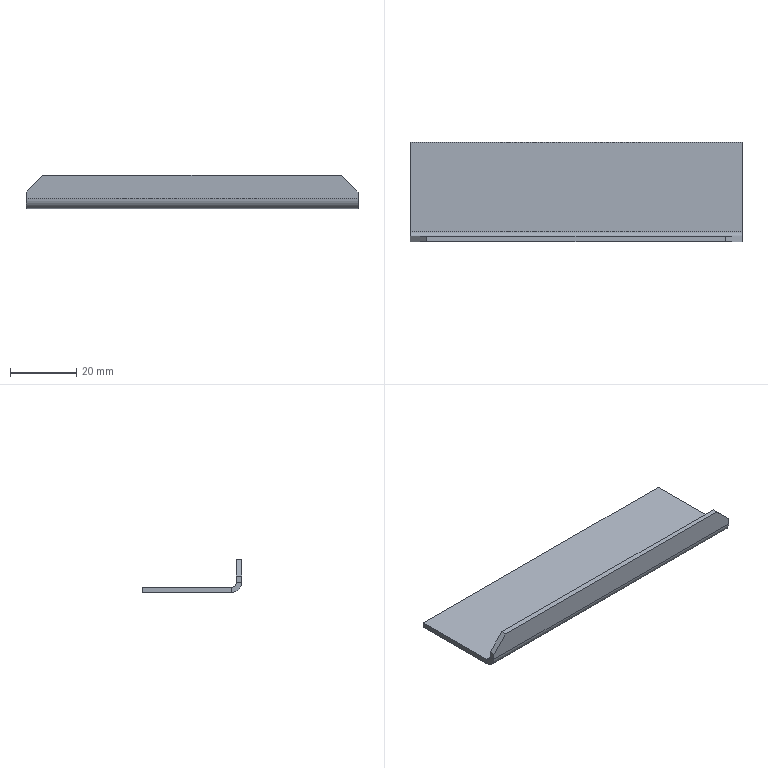Part | SolidWorks | features Chamfer 1, FlatPattern 1, SMBaseFlange 1, SheetMetal 1, UnFold 1 | 1 solid | 16 faces | box 100 x 30 x 10 mm | volume 5946 mm3 | plane 14 | cylinder 2 | commonest cylinder face diameters 3 x1 6.2 x1
STEP:
#1=CARTESIAN_POINT('',(50.,0.,3.1));
#2=VERTEX_POINT('',#1);
#3=CARTESIAN_POINT('',(50.,1.6,3.1));
#4=VERTEX_POINT('',#3);
#5=CARTESIAN_POINT('',(50.,0.,3.1));
#6=DIRECTION('',(0.,1.,0.));
#7=VECTOR('',#6,1000.);
#8=LINE('',#5,#7);
#9=EDGE_CURVE('',#2,#4,#8,.T.);
#10=ORIENTED_EDGE('',*,*,#9,.F.);
#11=CARTESIAN_POINT('',(50.,3.1,0.));
#12=VERTEX_POINT('',#11);
#13=CARTESIAN_POINT('',(50.,3.1,3.1));
#14=DIRECTION('',(1.,0.,0.));
#15=DIRECTION('',(0.,0.,1.));
#16=AXIS2_PLACEMENT_3D('',#13,#14,#15);
#17=CIRCLE('',#16,3.1);
#18=EDGE_CURVE('',#2,#12,#17,.T.);
#19=ORIENTED_EDGE('',*,*,#18,.T.);
#20=CARTESIAN_POINT('',(50.,3.1,1.6));
#21=VERTEX_POINT('',#20);
#22=CARTESIAN_POINT('',(50.,3.1,1.6));
#23=DIRECTION('',(0.,0.,-1.));
#24=VECTOR('',#23,1000.);
#25=LINE('',#22,#24);
#26=EDGE_CURVE('',#21,#12,#25,.T.);
#27=ORIENTED_EDGE('',*,*,#26,.F.);
#28=CARTESIAN_POINT('',(50.,3.1,3.1));
#29=DIRECTION('',(1.,0.,0.));
#30=DIRECTION('',(0.,0.,-1.));
#31=AXIS2_PLACEMENT_3D('',#28,#29,#30);
#32=CIRCLE('',#31,1.5);
#33=EDGE_CURVE('',#4,#21,#32,.T.);
#34=ORIENTED_EDGE('',*,*,#33,.F.);
#35=EDGE_LOOP('',(#10,#19,#27,#34));
#36=FACE_OUTER_BOUND('',#35,.T.);
#37=CARTESIAN_POINT('',(50.,0.,3.1));
#38=DIRECTION('',(1.,0.,0.));
#39=DIRECTION('',(0.,0.,-1.));
#40=AXIS2_PLACEMENT_3D('',#37,#38,#39);
#41=PLANE('',#40);
#42=ADVANCED_FACE('',(#36),#41,.T.);
#43=CARTESIAN_POINT('',(50.,1.6,5.));
#44=VERTEX_POINT('',#43);
#45=CARTESIAN_POINT('',(50.,1.6,0.));
#46=DIRECTION('',(0.,0.,-1.));
#47=VECTOR('',#46,1000.);
#48=LINE('',#45,#47);
#49=EDGE_CURVE('',#44,#4,#48,.T.);
#50=ORIENTED_EDGE('',*,*,#49,.F.);
#51=CARTESIAN_POINT('',(50.,0.,5.));
#52=VERTEX_POINT('',#51);
#53=CARTESIAN_POINT('',(50.,3.1,5.));
#54=DIRECTION('',(0.,-1.,0.));
#55=VECTOR('',#54,1000.);
#56=LINE('',#53,#55);
#57=EDGE_CURVE('',#44,#52,#56,.T.);
#58=ORIENTED_EDGE('',*,*,#57,.T.);
#59=CARTESIAN_POINT('',(50.,0.,0.));
#60=DIRECTION('',(0.,0.,-1.));
#61=VECTOR('',#60,1000.);
#62=LINE('',#59,#61);
#63=EDGE_CURVE('',#52,#2,#62,.T.);
#64=ORIENTED_EDGE('',*,*,#63,.T.);
#65=ORIENTED_EDGE('',*,*,#9,.T.);
#66=EDGE_LOOP('',(#50,#58,#64,#65));
#67=FACE_OUTER_BOUND('',#66,.T.);
#68=CARTESIAN_POINT('',(50.,3.1,1.6));
#69=DIRECTION('',(1.,0.,0.));
#70=DIRECTION('',(0.,0.,-1.));
#71=AXIS2_PLACEMENT_3D('',#68,#69,#70);
#72=PLANE('',#71);
#73=ADVANCED_FACE('',(#67),#72,.T.);
#74=CARTESIAN_POINT('',(-50.,3.1,0.));
#75=VERTEX_POINT('',#74);
#76=CARTESIAN_POINT('',(-50.,3.1,1.6));
#77=VERTEX_POINT('',#76);
#78=CARTESIAN_POINT('',(-50.,3.1,0.));
#79=DIRECTION('',(0.,0.,1.));
#80=VECTOR('',#79,1000.);
#81=LINE('',#78,#80);
#82=EDGE_CURVE('',#75,#77,#81,.T.);
#83=ORIENTED_EDGE('',*,*,#82,.F.);
#84=CARTESIAN_POINT('',(-50.,0.,3.1));
#85=VERTEX_POINT('',#84);
#86=CARTESIAN_POINT('',(-50.,3.1,3.1));
#87=DIRECTION('',(1.,0.,0.));
#88=DIRECTION('',(0.,0.,1.));
#89=AXIS2_PLACEMENT_3D('',#86,#87,#88);
#90=CIRCLE('',#89,3.1);
#91=EDGE_CURVE('',#85,#75,#90,.T.);
#92=ORIENTED_EDGE('',*,*,#91,.F.);
#93=CARTESIAN_POINT('',(-50.,1.6,3.1));
#94=VERTEX_POINT('',#93);
#95=CARTESIAN_POINT('',(-50.,1.6,3.1));
#96=DIRECTION('',(0.,-1.,0.));
#97=VECTOR('',#96,1000.);
#98=LINE('',#95,#97);
#99=EDGE_CURVE('',#94,#85,#98,.T.);
#100=ORIENTED_EDGE('',*,*,#99,.F.);
#101=CARTESIAN_POINT('',(-50.,3.1,3.1));
#102=DIRECTION('',(1.,0.,0.));
#103=DIRECTION('',(0.,0.,-1.));
#104=AXIS2_PLACEMENT_3D('',#101,#102,#103);
#105=CIRCLE('',#104,1.5);
#106=EDGE_CURVE('',#94,#77,#105,.T.);
#107=ORIENTED_EDGE('',*,*,#106,.T.);
#108=EDGE_LOOP('',(#83,#92,#100,#107));
#109=FACE_OUTER_BOUND('',#108,.T.);
#110=CARTESIAN_POINT('',(-50.,3.1,0.));
#111=DIRECTION('',(-1.,0.,0.));
#112=DIRECTION('',(0.,0.,1.));
#113=AXIS2_PLACEMENT_3D('',#110,#111,#112);
#114=PLANE('',#113);
#115=ADVANCED_FACE('',(#109),#114,.T.);
#116=CARTESIAN_POINT('',(-50.,30.,0.));
#117=VERTEX_POINT('',#116);
#118=CARTESIAN_POINT('',(-50.,0.,0.));
#119=DIRECTION('',(0.,1.,0.));
#120=VECTOR('',#119,1000.);
#121=LINE('',#118,#120);
#122=EDGE_CURVE('',#75,#117,#121,.T.);
#123=ORIENTED_EDGE('',*,*,#122,.F.);
#124=ORIENTED_EDGE('',*,*,#82,.T.);
#125=CARTESIAN_POINT('',(-50.,30.,1.6));
#126=VERTEX_POINT('',#125);
#127=CARTESIAN_POINT('',(-50.,0.,1.6));
#128=DIRECTION('',(0.,1.,0.));
#129=VECTOR('',#128,1000.);
#130=LINE('',#127,#129);
#131=EDGE_CURVE('',#77,#126,#130,.T.);
#132=ORIENTED_EDGE('',*,*,#131,.T.);
#133=CARTESIAN_POINT('',(-50.,30.,1.6));
#134=DIRECTION('',(0.,0.,-1.));
#135=VECTOR('',#134,1000.);
#136=LINE('',#133,#135);
#137=EDGE_CURVE('',#126,#117,#136,.T.);
#138=ORIENTED_EDGE('',*,*,#137,.T.);
#139=EDGE_LOOP('',(#123,#124,#132,#138));
#140=FACE_OUTER_BOUND('',#139,.T.);
#141=CARTESIAN_POINT('',(-50.,1.6,3.1));
#142=DIRECTION('',(-1.,0.,0.));
#143=DIRECTION('',(0.,0.,1.));
#144=AXIS2_PLACEMENT_3D('',#141,#142,#143);
#145=PLANE('',#144);
#146=ADVANCED_FACE('',(#140),#145,.T.);
#147=ORIENTED_EDGE('',*,*,#122,.T.);
#148=CARTESIAN_POINT('',(50.,30.,0.));
#149=VERTEX_POINT('',#148);
#150=CARTESIAN_POINT('',(50.,30.,0.));
#151=DIRECTION('',(-1.,0.,0.));
#152=VECTOR('',#151,1000.);
#153=LINE('',#150,#152);
#154=EDGE_CURVE('',#149,#117,#153,.T.);
#155=ORIENTED_EDGE('',*,*,#154,.F.);
#156=CARTESIAN_POINT('',(50.,0.,0.));
#157=DIRECTION('',(0.,1.,0.));
#158=VECTOR('',#157,1000.);
#159=LINE('',#156,#158);
#160=EDGE_CURVE('',#12,#149,#159,.T.);
#161=ORIENTED_EDGE('',*,*,#160,.F.);
#162=CARTESIAN_POINT('',(50.,3.1,0.));
#163=DIRECTION('',(-1.,0.,0.));
#164=VECTOR('',#163,1000.);
#165=LINE('',#162,#164);
#166=EDGE_CURVE('',#12,#75,#165,.T.);
#167=ORIENTED_EDGE('',*,*,#166,.T.);
#168=EDGE_LOOP('',(#147,#155,#161,#167));
#169=FACE_OUTER_BOUND('',#168,.T.);
#170=CARTESIAN_POINT('',(50.,0.,0.));
#171=DIRECTION('',(0.,0.,1.));
#172=DIRECTION('',(1.,0.,0.));
#173=AXIS2_PLACEMENT_3D('',#170,#171,#172);
#174=PLANE('',#173);
#175=ADVANCED_FACE('',(#169),#174,.F.);
#176=ORIENTED_EDGE('',*,*,#137,.F.);
#177=CARTESIAN_POINT('',(50.,30.,1.6));
#178=VERTEX_POINT('',#177);
#179=CARTESIAN_POINT('',(50.,30.,1.6));
#180=DIRECTION('',(-1.,0.,0.));
#181=VECTOR('',#180,1000.);
#182=LINE('',#179,#181);
#183=EDGE_CURVE('',#178,#126,#182,.T.);
#184=ORIENTED_EDGE('',*,*,#183,.F.);
#185=CARTESIAN_POINT('',(50.,30.,1.6));
#186=DIRECTION('',(0.,0.,-1.));
#187=VECTOR('',#186,1000.);
#188=LINE('',#185,#187);
#189=EDGE_CURVE('',#178,#149,#188,.T.);
#190=ORIENTED_EDGE('',*,*,#189,.T.);
#191=ORIENTED_EDGE('',*,*,#154,.T.);
#192=EDGE_LOOP('',(#176,#184,#190,#191));
#193=FACE_OUTER_BOUND('',#192,.T.);
#194=CARTESIAN_POINT('',(50.,30.,1.6));
#195=DIRECTION('',(0.,1.,0.));
#196=DIRECTION('',(0.,0.,1.));
#197=AXIS2_PLACEMENT_3D('',#194,#195,#196);
#198=PLANE('',#197);
#199=ADVANCED_FACE('',(#193),#198,.T.);
#200=ORIENTED_EDGE('',*,*,#131,.F.);
#201=CARTESIAN_POINT('',(50.,3.1,1.6));
#202=DIRECTION('',(-1.,0.,0.));
#203=VECTOR('',#202,1000.);
#204=LINE('',#201,#203);
#205=EDGE_CURVE('',#21,#77,#204,.T.);
#206=ORIENTED_EDGE('',*,*,#205,.F.);
#207=CARTESIAN_POINT('',(50.,0.,1.6));
#208=DIRECTION('',(0.,1.,0.));
#209=VECTOR('',#208,1000.);
#210=LINE('',#207,#209);
#211=EDGE_CURVE('',#21,#178,#210,.T.);
#212=ORIENTED_EDGE('',*,*,#211,.T.);
#213=ORIENTED_EDGE('',*,*,#183,.T.);
#214=EDGE_LOOP('',(#200,#206,#212,#213));
#215=FACE_OUTER_BOUND('',#214,.T.);
#216=CARTESIAN_POINT('',(50.,0.,1.6));
#217=DIRECTION('',(0.,0.,1.));
#218=DIRECTION('',(1.,0.,0.));
#219=AXIS2_PLACEMENT_3D('',#216,#217,#218);
#220=PLANE('',#219);
#221=ADVANCED_FACE('',(#215),#220,.T.);
#222=ORIENTED_EDGE('',*,*,#106,.F.);
#223=CARTESIAN_POINT('',(50.,1.6,3.1));
#224=DIRECTION('',(-1.,0.,0.));
#225=VECTOR('',#224,1000.);
#226=LINE('',#223,#225);
#227=EDGE_CURVE('',#4,#94,#226,.T.);
#228=ORIENTED_EDGE('',*,*,#227,.F.);
#229=ORIENTED_EDGE('',*,*,#33,.T.);
#230=ORIENTED_EDGE('',*,*,#205,.T.);
#231=EDGE_LOOP('',(#222,#228,#229,#230));
#232=FACE_OUTER_BOUND('',#231,.T.);
#233=CARTESIAN_POINT('',(50.,3.1,3.1));
#234=DIRECTION('',(-1.,0.,0.));
#235=DIRECTION('',(0.,0.,1.));
#236=AXIS2_PLACEMENT_3D('',#233,#234,#235);
#237=CYLINDRICAL_SURFACE('',#236,1.5);
#238=ADVANCED_FACE('',(#232),#237,.F.);
#239=CARTESIAN_POINT('',(-50.,1.6,5.));
#240=VERTEX_POINT('',#239);
#241=CARTESIAN_POINT('',(-50.,1.6,0.));
#242=DIRECTION('',(0.,0.,-1.));
#243=VECTOR('',#242,1000.);
#244=LINE('',#241,#243);
#245=EDGE_CURVE('',#240,#94,#244,.T.);
#246=ORIENTED_EDGE('',*,*,#245,.F.);
#247=CARTESIAN_POINT('',(-45.,1.6,10.));
#248=VERTEX_POINT('',#247);
#249=CARTESIAN_POINT('',(-2.5,1.6,52.5));
#250=DIRECTION('',(0.7071,0.,0.7071));
#251=VECTOR('',#250,1000.);
#252=LINE('',#249,#251);
#253=EDGE_CURVE('',#240,#248,#252,.T.);
#254=ORIENTED_EDGE('',*,*,#253,.T.);
#255=CARTESIAN_POINT('',(45.,1.6,10.));
#256=VERTEX_POINT('',#255);
#257=CARTESIAN_POINT('',(50.,1.6,10.));
#258=DIRECTION('',(-1.,0.,0.));
#259=VECTOR('',#258,1000.);
#260=LINE('',#257,#259);
#261=EDGE_CURVE('',#256,#248,#260,.T.);
#262=ORIENTED_EDGE('',*,*,#261,.F.);
#263=CARTESIAN_POINT('',(52.5,1.6,2.5));
#264=DIRECTION('',(0.7071,0.,-0.7071));
#265=VECTOR('',#264,1000.);
#266=LINE('',#263,#265);
#267=EDGE_CURVE('',#256,#44,#266,.T.);
#268=ORIENTED_EDGE('',*,*,#267,.T.);
#269=ORIENTED_EDGE('',*,*,#49,.T.);
#270=ORIENTED_EDGE('',*,*,#227,.T.);
#271=EDGE_LOOP('',(#246,#254,#262,#268,#269,#270));
#272=FACE_OUTER_BOUND('',#271,.T.);
#273=CARTESIAN_POINT('',(50.,1.6,0.));
#274=DIRECTION('',(0.,1.,0.));
#275=DIRECTION('',(0.,0.,1.));
#276=AXIS2_PLACEMENT_3D('',#273,#274,#275);
#277=PLANE('',#276);
#278=ADVANCED_FACE('',(#272),#277,.T.);
#279=ORIENTED_EDGE('',*,*,#261,.T.);
#280=CARTESIAN_POINT('',(-45.,0.,10.));
#281=VERTEX_POINT('',#280);
#282=CARTESIAN_POINT('',(-45.,0.,10.));
#283=DIRECTION('',(0.,-1.,0.));
#284=VECTOR('',#283,1000.);
#285=LINE('',#282,#284);
#286=EDGE_CURVE('',#248,#281,#285,.T.);
#287=ORIENTED_EDGE('',*,*,#286,.T.);
#288=CARTESIAN_POINT('',(45.,0.,10.));
#289=VERTEX_POINT('',#288);
#290=CARTESIAN_POINT('',(50.,0.,10.));
#291=DIRECTION('',(-1.,0.,0.));
#292=VECTOR('',#291,1000.);
#293=LINE('',#290,#292);
#294=EDGE_CURVE('',#289,#281,#293,.T.);
#295=ORIENTED_EDGE('',*,*,#294,.F.);
#296=CARTESIAN_POINT('',(45.,0.,10.));
#297=DIRECTION('',(0.,1.,0.));
#298=VECTOR('',#297,1000.);
#299=LINE('',#296,#298);
#300=EDGE_CURVE('',#289,#256,#299,.T.);
#301=ORIENTED_EDGE('',*,*,#300,.T.);
#302=EDGE_LOOP('',(#279,#287,#295,#301));
#303=FACE_OUTER_BOUND('',#302,.T.);
#304=CARTESIAN_POINT('',(50.,0.,10.));
#305=DIRECTION('',(0.,0.,1.));
#306=DIRECTION('',(1.,0.,0.));
#307=AXIS2_PLACEMENT_3D('',#304,#305,#306);
#308=PLANE('',#307);
#309=ADVANCED_FACE('',(#303),#308,.T.);
#310=ORIENTED_EDGE('',*,*,#294,.T.);
#311=CARTESIAN_POINT('',(-50.,0.,5.));
#312=VERTEX_POINT('',#311);
#313=CARTESIAN_POINT('',(-50.,0.,5.));
#314=DIRECTION('',(-0.7071,0.,-0.7071));
#315=VECTOR('',#314,1000.);
#316=LINE('',#313,#315);
#317=EDGE_CURVE('',#281,#312,#316,.T.);
#318=ORIENTED_EDGE('',*,*,#317,.T.);
#319=CARTESIAN_POINT('',(-50.,0.,0.));
#320=DIRECTION('',(0.,0.,-1.));
#321=VECTOR('',#320,1000.);
#322=LINE('',#319,#321);
#323=EDGE_CURVE('',#312,#85,#322,.T.);
#324=ORIENTED_EDGE('',*,*,#323,.T.);
#325=CARTESIAN_POINT('',(50.,0.,3.1));
#326=DIRECTION('',(-1.,0.,0.));
#327=VECTOR('',#326,1000.);
#328=LINE('',#325,#327);
#329=EDGE_CURVE('',#2,#85,#328,.T.);
#330=ORIENTED_EDGE('',*,*,#329,.F.);
#331=ORIENTED_EDGE('',*,*,#63,.F.);
#332=CARTESIAN_POINT('',(45.,0.,10.));
#333=DIRECTION('',(-0.7071,0.,0.7071));
#334=VECTOR('',#333,1000.);
#335=LINE('',#332,#334);
#336=EDGE_CURVE('',#52,#289,#335,.T.);
#337=ORIENTED_EDGE('',*,*,#336,.T.);
#338=EDGE_LOOP('',(#310,#318,#324,#330,#331,#337));
#339=FACE_OUTER_BOUND('',#338,.T.);
#340=CARTESIAN_POINT('',(50.,0.,0.));
#341=DIRECTION('',(0.,1.,0.));
#342=DIRECTION('',(0.,0.,1.));
#343=AXIS2_PLACEMENT_3D('',#340,#341,#342);
#344=PLANE('',#343);
#345=ADVANCED_FACE('',(#339),#344,.F.);
#346=ORIENTED_EDGE('',*,*,#91,.T.);
#347=ORIENTED_EDGE('',*,*,#166,.F.);
#348=ORIENTED_EDGE('',*,*,#18,.F.);
#349=ORIENTED_EDGE('',*,*,#329,.T.);
#350=EDGE_LOOP('',(#346,#347,#348,#349));
#351=FACE_OUTER_BOUND('',#350,.T.);
#352=CARTESIAN_POINT('',(50.,3.1,3.1));
#353=DIRECTION('',(-1.,0.,0.));
#354=DIRECTION('',(0.,0.,1.));
#355=AXIS2_PLACEMENT_3D('',#352,#353,#354);
#356=CYLINDRICAL_SURFACE('',#355,3.1);
#357=ADVANCED_FACE('',(#351),#356,.T.);
#358=ORIENTED_EDGE('',*,*,#160,.T.);
#359=ORIENTED_EDGE('',*,*,#189,.F.);
#360=ORIENTED_EDGE('',*,*,#211,.F.);
#361=ORIENTED_EDGE('',*,*,#26,.T.);
#362=EDGE_LOOP('',(#358,#359,#360,#361));
#363=FACE_OUTER_BOUND('',#362,.T.);
#364=CARTESIAN_POINT('',(50.,3.1,3.1));
#365=DIRECTION('',(1.,0.,0.));
#366=DIRECTION('',(0.,0.,-1.));
#367=AXIS2_PLACEMENT_3D('',#364,#365,#366);
#368=PLANE('',#367);
#369=ADVANCED_FACE('',(#363),#368,.T.);
#370=ORIENTED_EDGE('',*,*,#323,.F.);
#371=CARTESIAN_POINT('',(-50.,1.6,5.));
#372=DIRECTION('',(0.,1.,0.));
#373=VECTOR('',#372,1000.);
#374=LINE('',#371,#373);
#375=EDGE_CURVE('',#312,#240,#374,.T.);
#376=ORIENTED_EDGE('',*,*,#375,.T.);
#377=ORIENTED_EDGE('',*,*,#245,.T.);
#378=ORIENTED_EDGE('',*,*,#99,.T.);
#379=EDGE_LOOP('',(#370,#376,#377,#378));
#380=FACE_OUTER_BOUND('',#379,.T.);
#381=CARTESIAN_POINT('',(-50.,3.1,3.1));
#382=DIRECTION('',(1.,0.,0.));
#383=DIRECTION('',(0.,0.,-1.));
#384=AXIS2_PLACEMENT_3D('',#381,#382,#383);
#385=PLANE('',#384);
#386=ADVANCED_FACE('',(#380),#385,.F.);
#387=ORIENTED_EDGE('',*,*,#317,.F.);
#388=ORIENTED_EDGE('',*,*,#286,.F.);
#389=ORIENTED_EDGE('',*,*,#253,.F.);
#390=ORIENTED_EDGE('',*,*,#375,.F.);
#391=EDGE_LOOP('',(#387,#388,#389,#390));
#392=FACE_OUTER_BOUND('',#391,.T.);
#393=CARTESIAN_POINT('',(-50.,3.1,5.));
#394=DIRECTION('',(-0.7071,0.,0.7071));
#395=DIRECTION('',(0.,-1.,0.));
#396=AXIS2_PLACEMENT_3D('',#393,#394,#395);
#397=PLANE('',#396);
#398=ADVANCED_FACE('',(#392),#397,.T.);
#399=ORIENTED_EDGE('',*,*,#336,.F.);
#400=ORIENTED_EDGE('',*,*,#57,.F.);
#401=ORIENTED_EDGE('',*,*,#267,.F.);
#402=ORIENTED_EDGE('',*,*,#300,.F.);
#403=EDGE_LOOP('',(#399,#400,#401,#402));
#404=FACE_OUTER_BOUND('',#403,.T.);
#405=CARTESIAN_POINT('',(45.,0.,10.));
#406=DIRECTION('',(-0.7071,0.,-0.7071));
#407=DIRECTION('',(0.,1.,0.));
#408=AXIS2_PLACEMENT_3D('',#405,#406,#407);
#409=PLANE('',#408);
#410=ADVANCED_FACE('',(#404),#409,.F.);
#411=CLOSED_SHELL('',(#42,#73,#115,#146,#175,#199,#221,#238,#278,#309,#345,#357,#369,#386,#398,#410));
#412=MANIFOLD_SOLID_BREP('',#411);
#413=CARTESIAN_POINT('',(0.,0.,0.));
#414=DIRECTION('',(0.,0.,1.));
#415=DIRECTION('',(1.,0.,0.));
#416=AXIS2_PLACEMENT_3D('',#413,#414,#415);
#417=(LENGTH_UNIT()NAMED_UNIT(*)SI_UNIT(.MILLI.,.METRE.));
#418=UNCERTAINTY_MEASURE_WITH_UNIT(LENGTH_MEASURE(0.00001),#417,'','');
#419=(NAMED_UNIT(*)PLANE_ANGLE_UNIT()SI_UNIT($,.RADIAN.));
#420=(NAMED_UNIT(*)SI_UNIT($,.STERADIAN.)SOLID_ANGLE_UNIT());
#421=(GEOMETRIC_REPRESENTATION_CONTEXT(3)GLOBAL_UNCERTAINTY_ASSIGNED_CONTEXT((#418))GLOBAL_UNIT_ASSIGNED_CONTEXT((#417,#419,#420))REPRESENTATION_CONTEXT('',''));
#422=ADVANCED_BREP_SHAPE_REPRESENTATION('',(#412,#416),#421);